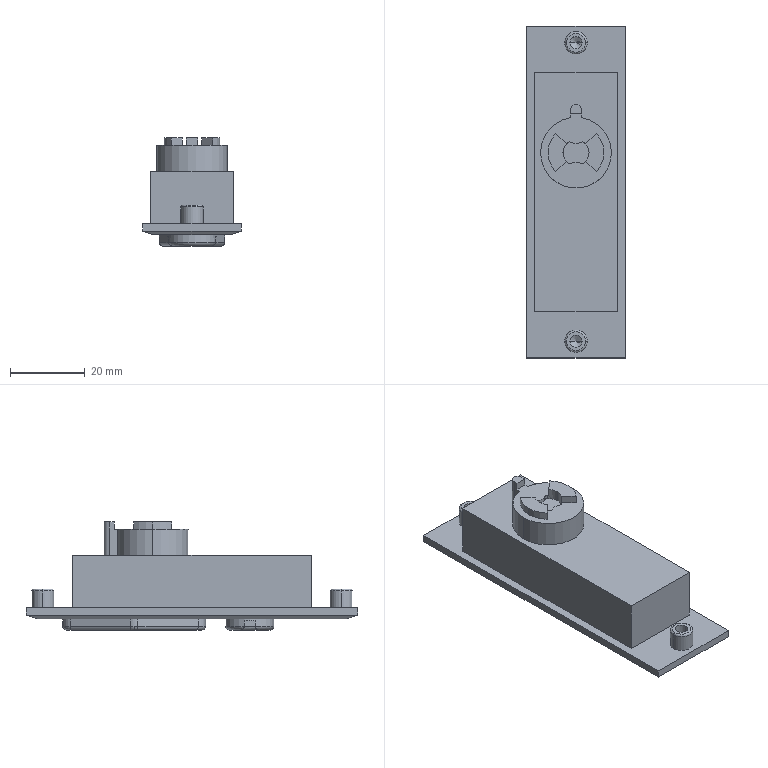Part | SolidWorks | features ICE 11, Fillet 3, Chamfer 1, Extrusion 1, HoleWzd 1 | 1 solid | 99 faces | box 26.5 x 89 x 29 mm | volume 30365 mm3 | plane 43 | cylinder 41 | torus 11 | cone 4 | commonest cylinder face diameters 2 x14 6 x9 3.3 x4 7 x3 15 x3 19 x3